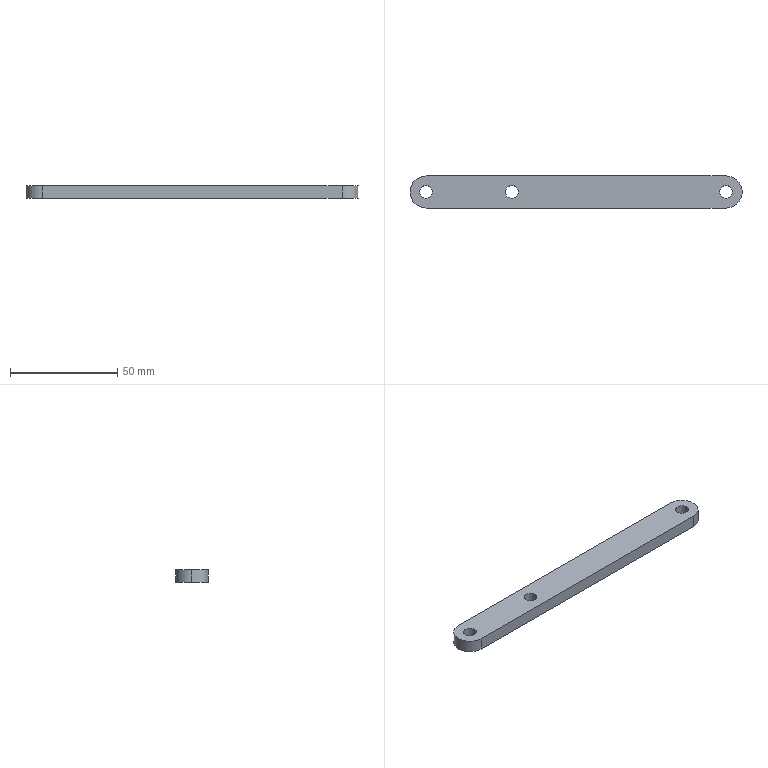Part | SolidWorks | features Extrusion 1 | 1 solid | 13 faces | box 155 x 15 x 6 mm | volume 13151 mm3 | cylinder 9 | plane 4 | commonest cylinder face diameters 6 x6 15 x3
STEP:
#1=CARTESIAN_POINT('',(137.,0.,6.));
#2=VERTEX_POINT('',#1);
#3=CARTESIAN_POINT('',(143.,0.,6.));
#4=VERTEX_POINT('',#3);
#5=CARTESIAN_POINT('',(140.,0.,6.));
#6=DIRECTION('',(0.,0.,1.));
#7=DIRECTION('',(1.,0.,0.));
#8=AXIS2_PLACEMENT_3D('',#5,#6,#7);
#9=CIRCLE('',#8,3.);
#10=EDGE_CURVE('',#2,#4,#9,.T.);
#11=ORIENTED_EDGE('',*,*,#10,.T.);
#12=CARTESIAN_POINT('',(143.,0.,0.));
#13=VERTEX_POINT('',#12);
#14=CARTESIAN_POINT('',(143.,0.,6.));
#15=DIRECTION('',(0.,0.,-1.));
#16=VECTOR('',#15,1000.);
#17=LINE('',#14,#16);
#18=EDGE_CURVE('',#4,#13,#17,.T.);
#19=ORIENTED_EDGE('',*,*,#18,.T.);
#20=CARTESIAN_POINT('',(137.,0.,0.));
#21=VERTEX_POINT('',#20);
#22=CARTESIAN_POINT('',(140.,0.,0.));
#23=DIRECTION('',(0.,0.,1.));
#24=DIRECTION('',(1.,0.,0.));
#25=AXIS2_PLACEMENT_3D('',#22,#23,#24);
#26=CIRCLE('',#25,3.);
#27=EDGE_CURVE('',#21,#13,#26,.T.);
#28=ORIENTED_EDGE('',*,*,#27,.F.);
#29=CARTESIAN_POINT('',(137.,0.,6.));
#30=DIRECTION('',(0.,0.,-1.));
#31=VECTOR('',#30,1000.);
#32=LINE('',#29,#31);
#33=EDGE_CURVE('',#2,#21,#32,.T.);
#34=ORIENTED_EDGE('',*,*,#33,.F.);
#35=EDGE_LOOP('',(#11,#19,#28,#34));
#36=FACE_OUTER_BOUND('',#35,.T.);
#37=CARTESIAN_POINT('',(140.,0.,6.));
#38=DIRECTION('',(0.,0.,-1.));
#39=DIRECTION('',(-1.,0.,0.));
#40=AXIS2_PLACEMENT_3D('',#37,#38,#39);
#41=CYLINDRICAL_SURFACE('',#40,3.);
#42=ADVANCED_FACE('',(#36),#41,.F.);
#43=CARTESIAN_POINT('',(37.,0.,6.));
#44=VERTEX_POINT('',#43);
#45=CARTESIAN_POINT('',(43.,0.,6.));
#46=VERTEX_POINT('',#45);
#47=CARTESIAN_POINT('',(40.,0.,6.));
#48=DIRECTION('',(0.,0.,1.));
#49=DIRECTION('',(1.,0.,0.));
#50=AXIS2_PLACEMENT_3D('',#47,#48,#49);
#51=CIRCLE('',#50,3.);
#52=EDGE_CURVE('',#44,#46,#51,.T.);
#53=ORIENTED_EDGE('',*,*,#52,.T.);
#54=CARTESIAN_POINT('',(43.,0.,0.));
#55=VERTEX_POINT('',#54);
#56=CARTESIAN_POINT('',(43.,0.,6.));
#57=DIRECTION('',(0.,0.,-1.));
#58=VECTOR('',#57,1000.);
#59=LINE('',#56,#58);
#60=EDGE_CURVE('',#46,#55,#59,.T.);
#61=ORIENTED_EDGE('',*,*,#60,.T.);
#62=CARTESIAN_POINT('',(37.,0.,0.));
#63=VERTEX_POINT('',#62);
#64=CARTESIAN_POINT('',(40.,0.,0.));
#65=DIRECTION('',(0.,0.,1.));
#66=DIRECTION('',(1.,0.,0.));
#67=AXIS2_PLACEMENT_3D('',#64,#65,#66);
#68=CIRCLE('',#67,3.);
#69=EDGE_CURVE('',#63,#55,#68,.T.);
#70=ORIENTED_EDGE('',*,*,#69,.F.);
#71=CARTESIAN_POINT('',(37.,0.,6.));
#72=DIRECTION('',(0.,0.,-1.));
#73=VECTOR('',#72,1000.);
#74=LINE('',#71,#73);
#75=EDGE_CURVE('',#44,#63,#74,.T.);
#76=ORIENTED_EDGE('',*,*,#75,.F.);
#77=EDGE_LOOP('',(#53,#61,#70,#76));
#78=FACE_OUTER_BOUND('',#77,.T.);
#79=CARTESIAN_POINT('',(40.,0.,6.));
#80=DIRECTION('',(0.,0.,-1.));
#81=DIRECTION('',(-1.,0.,0.));
#82=AXIS2_PLACEMENT_3D('',#79,#80,#81);
#83=CYLINDRICAL_SURFACE('',#82,3.);
#84=ADVANCED_FACE('',(#78),#83,.F.);
#85=CARTESIAN_POINT('',(-3.,0.,6.));
#86=VERTEX_POINT('',#85);
#87=CARTESIAN_POINT('',(3.,0.,6.));
#88=VERTEX_POINT('',#87);
#89=CARTESIAN_POINT('',(0.,0.,6.));
#90=DIRECTION('',(0.,0.,1.));
#91=DIRECTION('',(1.,0.,0.));
#92=AXIS2_PLACEMENT_3D('',#89,#90,#91);
#93=CIRCLE('',#92,3.);
#94=EDGE_CURVE('',#86,#88,#93,.T.);
#95=ORIENTED_EDGE('',*,*,#94,.T.);
#96=CARTESIAN_POINT('',(3.,0.,0.));
#97=VERTEX_POINT('',#96);
#98=CARTESIAN_POINT('',(3.,0.,6.));
#99=DIRECTION('',(0.,0.,-1.));
#100=VECTOR('',#99,1000.);
#101=LINE('',#98,#100);
#102=EDGE_CURVE('',#88,#97,#101,.T.);
#103=ORIENTED_EDGE('',*,*,#102,.T.);
#104=CARTESIAN_POINT('',(-3.,0.,0.));
#105=VERTEX_POINT('',#104);
#106=CARTESIAN_POINT('',(0.,0.,0.));
#107=DIRECTION('',(0.,0.,1.));
#108=DIRECTION('',(1.,0.,0.));
#109=AXIS2_PLACEMENT_3D('',#106,#107,#108);
#110=CIRCLE('',#109,3.);
#111=EDGE_CURVE('',#105,#97,#110,.T.);
#112=ORIENTED_EDGE('',*,*,#111,.F.);
#113=CARTESIAN_POINT('',(-3.,0.,6.));
#114=DIRECTION('',(0.,0.,-1.));
#115=VECTOR('',#114,1000.);
#116=LINE('',#113,#115);
#117=EDGE_CURVE('',#86,#105,#116,.T.);
#118=ORIENTED_EDGE('',*,*,#117,.F.);
#119=EDGE_LOOP('',(#95,#103,#112,#118));
#120=FACE_OUTER_BOUND('',#119,.T.);
#121=CARTESIAN_POINT('',(0.,0.,6.));
#122=DIRECTION('',(0.,0.,-1.));
#123=DIRECTION('',(-1.,0.,0.));
#124=AXIS2_PLACEMENT_3D('',#121,#122,#123);
#125=CYLINDRICAL_SURFACE('',#124,3.);
#126=ADVANCED_FACE('',(#120),#125,.F.);
#127=CARTESIAN_POINT('',(-7.5,0.,6.));
#128=VERTEX_POINT('',#127);
#129=CARTESIAN_POINT('',(0.,-7.5,6.));
#130=VERTEX_POINT('',#129);
#131=CARTESIAN_POINT('',(0.,0.,6.));
#132=DIRECTION('',(0.,0.,1.));
#133=DIRECTION('',(1.,0.,0.));
#134=AXIS2_PLACEMENT_3D('',#131,#132,#133);
#135=CIRCLE('',#134,7.5);
#136=EDGE_CURVE('',#128,#130,#135,.T.);
#137=ORIENTED_EDGE('',*,*,#136,.F.);
#138=CARTESIAN_POINT('',(-7.5,0.,0.));
#139=VERTEX_POINT('',#138);
#140=CARTESIAN_POINT('',(-7.5,0.,6.));
#141=DIRECTION('',(0.,0.,-1.));
#142=VECTOR('',#141,1000.);
#143=LINE('',#140,#142);
#144=EDGE_CURVE('',#128,#139,#143,.T.);
#145=ORIENTED_EDGE('',*,*,#144,.T.);
#146=CARTESIAN_POINT('',(0.,-7.5,0.));
#147=VERTEX_POINT('',#146);
#148=CARTESIAN_POINT('',(0.,0.,0.));
#149=DIRECTION('',(0.,0.,1.));
#150=DIRECTION('',(1.,0.,0.));
#151=AXIS2_PLACEMENT_3D('',#148,#149,#150);
#152=CIRCLE('',#151,7.5);
#153=EDGE_CURVE('',#139,#147,#152,.T.);
#154=ORIENTED_EDGE('',*,*,#153,.T.);
#155=CARTESIAN_POINT('',(0.,-7.5,6.));
#156=DIRECTION('',(0.,0.,-1.));
#157=VECTOR('',#156,1000.);
#158=LINE('',#155,#157);
#159=EDGE_CURVE('',#130,#147,#158,.T.);
#160=ORIENTED_EDGE('',*,*,#159,.F.);
#161=EDGE_LOOP('',(#137,#145,#154,#160));
#162=FACE_OUTER_BOUND('',#161,.T.);
#163=CARTESIAN_POINT('',(0.,0.,6.));
#164=DIRECTION('',(0.,0.,-1.));
#165=DIRECTION('',(-1.,0.,0.));
#166=AXIS2_PLACEMENT_3D('',#163,#164,#165);
#167=CYLINDRICAL_SURFACE('',#166,7.5);
#168=ADVANCED_FACE('',(#162),#167,.T.);
#169=ORIENTED_EDGE('',*,*,#52,.F.);
#170=CARTESIAN_POINT('',(40.,0.,6.));
#171=DIRECTION('',(0.,0.,1.));
#172=DIRECTION('',(1.,0.,0.));
#173=AXIS2_PLACEMENT_3D('',#170,#171,#172);
#174=CIRCLE('',#173,3.);
#175=EDGE_CURVE('',#46,#44,#174,.T.);
#176=ORIENTED_EDGE('',*,*,#175,.F.);
#177=EDGE_LOOP('',(#169,#176));
#178=FACE_BOUND('',#177,.T.);
#179=CARTESIAN_POINT('',(0.,7.5,6.));
#180=VERTEX_POINT('',#179);
#181=CARTESIAN_POINT('',(0.,0.,6.));
#182=DIRECTION('',(0.,0.,1.));
#183=DIRECTION('',(1.,0.,0.));
#184=AXIS2_PLACEMENT_3D('',#181,#182,#183);
#185=CIRCLE('',#184,7.5);
#186=EDGE_CURVE('',#180,#128,#185,.T.);
#187=ORIENTED_EDGE('',*,*,#186,.T.);
#188=ORIENTED_EDGE('',*,*,#136,.T.);
#189=CARTESIAN_POINT('',(140.,-7.5,6.));
#190=VERTEX_POINT('',#189);
#191=CARTESIAN_POINT('',(0.,-7.5,6.));
#192=DIRECTION('',(1.,0.,0.));
#193=VECTOR('',#192,1000.);
#194=LINE('',#191,#193);
#195=EDGE_CURVE('',#130,#190,#194,.T.);
#196=ORIENTED_EDGE('',*,*,#195,.T.);
#197=CARTESIAN_POINT('',(140.,7.5,6.));
#198=VERTEX_POINT('',#197);
#199=CARTESIAN_POINT('',(140.,0.,6.));
#200=DIRECTION('',(0.,0.,1.));
#201=DIRECTION('',(1.,0.,0.));
#202=AXIS2_PLACEMENT_3D('',#199,#200,#201);
#203=CIRCLE('',#202,7.5);
#204=EDGE_CURVE('',#190,#198,#203,.T.);
#205=ORIENTED_EDGE('',*,*,#204,.T.);
#206=CARTESIAN_POINT('',(0.,7.5,6.));
#207=DIRECTION('',(-1.,0.,0.));
#208=VECTOR('',#207,1000.);
#209=LINE('',#206,#208);
#210=EDGE_CURVE('',#198,#180,#209,.T.);
#211=ORIENTED_EDGE('',*,*,#210,.T.);
#212=EDGE_LOOP('',(#187,#188,#196,#205,#211));
#213=FACE_OUTER_BOUND('',#212,.T.);
#214=ORIENTED_EDGE('',*,*,#94,.F.);
#215=CARTESIAN_POINT('',(0.,0.,6.));
#216=DIRECTION('',(0.,0.,1.));
#217=DIRECTION('',(1.,0.,0.));
#218=AXIS2_PLACEMENT_3D('',#215,#216,#217);
#219=CIRCLE('',#218,3.);
#220=EDGE_CURVE('',#88,#86,#219,.T.);
#221=ORIENTED_EDGE('',*,*,#220,.F.);
#222=EDGE_LOOP('',(#214,#221));
#223=FACE_BOUND('',#222,.T.);
#224=ORIENTED_EDGE('',*,*,#10,.F.);
#225=CARTESIAN_POINT('',(140.,0.,6.));
#226=DIRECTION('',(0.,0.,1.));
#227=DIRECTION('',(1.,0.,0.));
#228=AXIS2_PLACEMENT_3D('',#225,#226,#227);
#229=CIRCLE('',#228,3.);
#230=EDGE_CURVE('',#4,#2,#229,.T.);
#231=ORIENTED_EDGE('',*,*,#230,.F.);
#232=EDGE_LOOP('',(#224,#231));
#233=FACE_BOUND('',#232,.T.);
#234=CARTESIAN_POINT('',(0.,0.,6.));
#235=DIRECTION('',(0.,0.,1.));
#236=DIRECTION('',(1.,0.,0.));
#237=AXIS2_PLACEMENT_3D('',#234,#235,#236);
#238=PLANE('',#237);
#239=ADVANCED_FACE('',(#178,#213,#223,#233),#238,.T.);
#240=CARTESIAN_POINT('',(0.,7.5,0.));
#241=VERTEX_POINT('',#240);
#242=CARTESIAN_POINT('',(0.,0.,0.));
#243=DIRECTION('',(0.,0.,1.));
#244=DIRECTION('',(1.,0.,0.));
#245=AXIS2_PLACEMENT_3D('',#242,#243,#244);
#246=CIRCLE('',#245,7.5);
#247=EDGE_CURVE('',#241,#139,#246,.T.);
#248=ORIENTED_EDGE('',*,*,#247,.F.);
#249=CARTESIAN_POINT('',(140.,7.5,0.));
#250=VERTEX_POINT('',#249);
#251=CARTESIAN_POINT('',(0.,7.5,0.));
#252=DIRECTION('',(-1.,0.,0.));
#253=VECTOR('',#252,1000.);
#254=LINE('',#251,#253);
#255=EDGE_CURVE('',#250,#241,#254,.T.);
#256=ORIENTED_EDGE('',*,*,#255,.F.);
#257=CARTESIAN_POINT('',(140.,-7.5,0.));
#258=VERTEX_POINT('',#257);
#259=CARTESIAN_POINT('',(140.,0.,0.));
#260=DIRECTION('',(0.,0.,1.));
#261=DIRECTION('',(1.,0.,0.));
#262=AXIS2_PLACEMENT_3D('',#259,#260,#261);
#263=CIRCLE('',#262,7.5);
#264=EDGE_CURVE('',#258,#250,#263,.T.);
#265=ORIENTED_EDGE('',*,*,#264,.F.);
#266=CARTESIAN_POINT('',(0.,-7.5,0.));
#267=DIRECTION('',(1.,0.,0.));
#268=VECTOR('',#267,1000.);
#269=LINE('',#266,#268);
#270=EDGE_CURVE('',#147,#258,#269,.T.);
#271=ORIENTED_EDGE('',*,*,#270,.F.);
#272=ORIENTED_EDGE('',*,*,#153,.F.);
#273=EDGE_LOOP('',(#248,#256,#265,#271,#272));
#274=FACE_OUTER_BOUND('',#273,.T.);
#275=ORIENTED_EDGE('',*,*,#111,.T.);
#276=CARTESIAN_POINT('',(0.,0.,0.));
#277=DIRECTION('',(0.,0.,1.));
#278=DIRECTION('',(1.,0.,0.));
#279=AXIS2_PLACEMENT_3D('',#276,#277,#278);
#280=CIRCLE('',#279,3.);
#281=EDGE_CURVE('',#97,#105,#280,.T.);
#282=ORIENTED_EDGE('',*,*,#281,.T.);
#283=EDGE_LOOP('',(#275,#282));
#284=FACE_BOUND('',#283,.T.);
#285=ORIENTED_EDGE('',*,*,#69,.T.);
#286=CARTESIAN_POINT('',(40.,0.,0.));
#287=DIRECTION('',(0.,0.,1.));
#288=DIRECTION('',(1.,0.,0.));
#289=AXIS2_PLACEMENT_3D('',#286,#287,#288);
#290=CIRCLE('',#289,3.);
#291=EDGE_CURVE('',#55,#63,#290,.T.);
#292=ORIENTED_EDGE('',*,*,#291,.T.);
#293=EDGE_LOOP('',(#285,#292));
#294=FACE_BOUND('',#293,.T.);
#295=ORIENTED_EDGE('',*,*,#27,.T.);
#296=CARTESIAN_POINT('',(140.,0.,0.));
#297=DIRECTION('',(0.,0.,1.));
#298=DIRECTION('',(1.,0.,0.));
#299=AXIS2_PLACEMENT_3D('',#296,#297,#298);
#300=CIRCLE('',#299,3.);
#301=EDGE_CURVE('',#13,#21,#300,.T.);
#302=ORIENTED_EDGE('',*,*,#301,.T.);
#303=EDGE_LOOP('',(#295,#302));
#304=FACE_BOUND('',#303,.T.);
#305=CARTESIAN_POINT('',(0.,0.,0.));
#306=DIRECTION('',(0.,0.,1.));
#307=DIRECTION('',(1.,0.,0.));
#308=AXIS2_PLACEMENT_3D('',#305,#306,#307);
#309=PLANE('',#308);
#310=ADVANCED_FACE('',(#274,#284,#294,#304),#309,.F.);
#311=ORIENTED_EDGE('',*,*,#144,.F.);
#312=ORIENTED_EDGE('',*,*,#186,.F.);
#313=CARTESIAN_POINT('',(0.,7.5,6.));
#314=DIRECTION('',(0.,0.,-1.));
#315=VECTOR('',#314,1000.);
#316=LINE('',#313,#315);
#317=EDGE_CURVE('',#180,#241,#316,.T.);
#318=ORIENTED_EDGE('',*,*,#317,.T.);
#319=ORIENTED_EDGE('',*,*,#247,.T.);
#320=EDGE_LOOP('',(#311,#312,#318,#319));
#321=FACE_OUTER_BOUND('',#320,.T.);
#322=CARTESIAN_POINT('',(0.,0.,6.));
#323=DIRECTION('',(0.,0.,-1.));
#324=DIRECTION('',(-1.,0.,0.));
#325=AXIS2_PLACEMENT_3D('',#322,#323,#324);
#326=CYLINDRICAL_SURFACE('',#325,7.5);
#327=ADVANCED_FACE('',(#321),#326,.T.);
#328=ORIENTED_EDGE('',*,*,#270,.T.);
#329=CARTESIAN_POINT('',(140.,-7.5,6.));
#330=DIRECTION('',(0.,0.,-1.));
#331=VECTOR('',#330,1000.);
#332=LINE('',#329,#331);
#333=EDGE_CURVE('',#190,#258,#332,.T.);
#334=ORIENTED_EDGE('',*,*,#333,.F.);
#335=ORIENTED_EDGE('',*,*,#195,.F.);
#336=ORIENTED_EDGE('',*,*,#159,.T.);
#337=EDGE_LOOP('',(#328,#334,#335,#336));
#338=FACE_OUTER_BOUND('',#337,.T.);
#339=CARTESIAN_POINT('',(0.,-7.5,6.));
#340=DIRECTION('',(0.,1.,0.));
#341=DIRECTION('',(-1.,0.,0.));
#342=AXIS2_PLACEMENT_3D('',#339,#340,#341);
#343=PLANE('',#342);
#344=ADVANCED_FACE('',(#338),#343,.F.);
#345=ORIENTED_EDGE('',*,*,#264,.T.);
#346=CARTESIAN_POINT('',(140.,7.5,6.));
#347=DIRECTION('',(0.,0.,-1.));
#348=VECTOR('',#347,1000.);
#349=LINE('',#346,#348);
#350=EDGE_CURVE('',#198,#250,#349,.T.);
#351=ORIENTED_EDGE('',*,*,#350,.F.);
#352=ORIENTED_EDGE('',*,*,#204,.F.);
#353=ORIENTED_EDGE('',*,*,#333,.T.);
#354=EDGE_LOOP('',(#345,#351,#352,#353));
#355=FACE_OUTER_BOUND('',#354,.T.);
#356=CARTESIAN_POINT('',(140.,0.,6.));
#357=DIRECTION('',(0.,0.,-1.));
#358=DIRECTION('',(-1.,0.,0.));
#359=AXIS2_PLACEMENT_3D('',#356,#357,#358);
#360=CYLINDRICAL_SURFACE('',#359,7.5);
#361=ADVANCED_FACE('',(#355),#360,.T.);
#362=ORIENTED_EDGE('',*,*,#255,.T.);
#363=ORIENTED_EDGE('',*,*,#317,.F.);
#364=ORIENTED_EDGE('',*,*,#210,.F.);
#365=ORIENTED_EDGE('',*,*,#350,.T.);
#366=EDGE_LOOP('',(#362,#363,#364,#365));
#367=FACE_OUTER_BOUND('',#366,.T.);
#368=CARTESIAN_POINT('',(0.,7.5,6.));
#369=DIRECTION('',(0.,-1.,0.));
#370=DIRECTION('',(1.,0.,0.));
#371=AXIS2_PLACEMENT_3D('',#368,#369,#370);
#372=PLANE('',#371);
#373=ADVANCED_FACE('',(#367),#372,.F.);
#374=ORIENTED_EDGE('',*,*,#102,.F.);
#375=ORIENTED_EDGE('',*,*,#220,.T.);
#376=ORIENTED_EDGE('',*,*,#117,.T.);
#377=ORIENTED_EDGE('',*,*,#281,.F.);
#378=EDGE_LOOP('',(#374,#375,#376,#377));
#379=FACE_OUTER_BOUND('',#378,.T.);
#380=CARTESIAN_POINT('',(0.,0.,6.));
#381=DIRECTION('',(0.,0.,-1.));
#382=DIRECTION('',(-1.,0.,0.));
#383=AXIS2_PLACEMENT_3D('',#380,#381,#382);
#384=CYLINDRICAL_SURFACE('',#383,3.);
#385=ADVANCED_FACE('',(#379),#384,.F.);
#386=ORIENTED_EDGE('',*,*,#60,.F.);
#387=ORIENTED_EDGE('',*,*,#175,.T.);
#388=ORIENTED_EDGE('',*,*,#75,.T.);
#389=ORIENTED_EDGE('',*,*,#291,.F.);
#390=EDGE_LOOP('',(#386,#387,#388,#389));
#391=FACE_OUTER_BOUND('',#390,.T.);
#392=CARTESIAN_POINT('',(40.,0.,6.));
#393=DIRECTION('',(0.,0.,-1.));
#394=DIRECTION('',(-1.,0.,0.));
#395=AXIS2_PLACEMENT_3D('',#392,#393,#394);
#396=CYLINDRICAL_SURFACE('',#395,3.);
#397=ADVANCED_FACE('',(#391),#396,.F.);
#398=ORIENTED_EDGE('',*,*,#18,.F.);
#399=ORIENTED_EDGE('',*,*,#230,.T.);
#400=ORIENTED_EDGE('',*,*,#33,.T.);
#401=ORIENTED_EDGE('',*,*,#301,.F.);
#402=EDGE_LOOP('',(#398,#399,#400,#401));
#403=FACE_OUTER_BOUND('',#402,.T.);
#404=CARTESIAN_POINT('',(140.,0.,6.));
#405=DIRECTION('',(0.,0.,-1.));
#406=DIRECTION('',(-1.,0.,0.));
#407=AXIS2_PLACEMENT_3D('',#404,#405,#406);
#408=CYLINDRICAL_SURFACE('',#407,3.);
#409=ADVANCED_FACE('',(#403),#408,.F.);
#410=CLOSED_SHELL('',(#42,#84,#126,#168,#239,#310,#327,#344,#361,#373,#385,#397,#409));
#411=MANIFOLD_SOLID_BREP('',#410);
#412=CARTESIAN_POINT('',(0.,0.,0.));
#413=DIRECTION('',(0.,0.,1.));
#414=DIRECTION('',(1.,0.,0.));
#415=AXIS2_PLACEMENT_3D('',#412,#413,#414);
#416=(LENGTH_UNIT()NAMED_UNIT(*)SI_UNIT(.MILLI.,.METRE.));
#417=UNCERTAINTY_MEASURE_WITH_UNIT(LENGTH_MEASURE(0.00001),#416,'','');
#418=(NAMED_UNIT(*)PLANE_ANGLE_UNIT()SI_UNIT($,.RADIAN.));
#419=(NAMED_UNIT(*)SI_UNIT($,.STERADIAN.)SOLID_ANGLE_UNIT());
#420=(GEOMETRIC_REPRESENTATION_CONTEXT(3)GLOBAL_UNCERTAINTY_ASSIGNED_CONTEXT((#417))GLOBAL_UNIT_ASSIGNED_CONTEXT((#416,#418,#419))REPRESENTATION_CONTEXT('',''));
#421=ADVANCED_BREP_SHAPE_REPRESENTATION('',(#411,#415),#420);